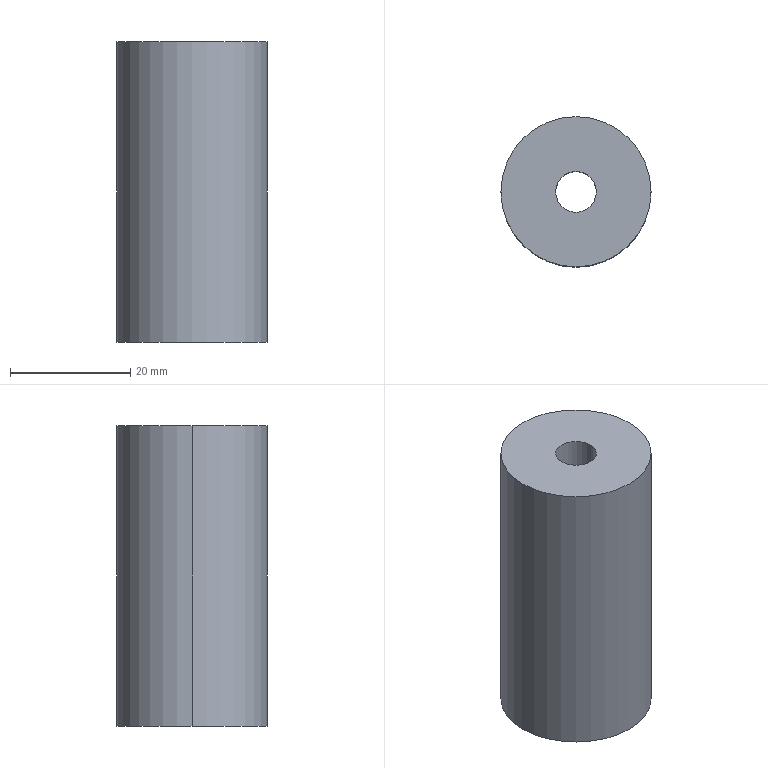Part | 1 solid | 6 faces | box 25 x 25 x 50 mm | volume 22728 mm3 | cylinder 4 | plane 2 | commonest cylinder face diameters 6.8 x2 25 x2
STEP:
#1=CARTESIAN_POINT('',(-3.4,0.,0.));
#2=VERTEX_POINT('',#1);
#3=CARTESIAN_POINT('',(3.4,0.,0.));
#4=VERTEX_POINT('',#3);
#5=CARTESIAN_POINT('',(0.,0.,0.));
#6=DIRECTION('',(0.,0.,1.));
#7=DIRECTION('',(1.,0.,0.));
#8=AXIS2_PLACEMENT_3D('',#5,#6,#7);
#9=CIRCLE('',#8,3.4);
#10=EDGE_CURVE('',#2,#4,#9,.T.);
#11=ORIENTED_EDGE('',*,*,#10,.F.);
#12=CARTESIAN_POINT('',(-3.4,0.,50.));
#13=VERTEX_POINT('',#12);
#14=CARTESIAN_POINT('',(-3.4,0.,50.));
#15=DIRECTION('',(0.,0.,1.));
#16=VECTOR('',#15,1000.);
#17=LINE('',#14,#16);
#18=EDGE_CURVE('',#2,#13,#17,.T.);
#19=ORIENTED_EDGE('',*,*,#18,.T.);
#20=CARTESIAN_POINT('',(3.4,0.,50.));
#21=VERTEX_POINT('',#20);
#22=CARTESIAN_POINT('',(0.,0.,50.));
#23=DIRECTION('',(0.,0.,1.));
#24=DIRECTION('',(1.,0.,0.));
#25=AXIS2_PLACEMENT_3D('',#22,#23,#24);
#26=CIRCLE('',#25,3.4);
#27=EDGE_CURVE('',#13,#21,#26,.T.);
#28=ORIENTED_EDGE('',*,*,#27,.T.);
#29=CARTESIAN_POINT('',(3.4,0.,50.));
#30=DIRECTION('',(0.,0.,1.));
#31=VECTOR('',#30,1000.);
#32=LINE('',#29,#31);
#33=EDGE_CURVE('',#4,#21,#32,.T.);
#34=ORIENTED_EDGE('',*,*,#33,.F.);
#35=EDGE_LOOP('',(#11,#19,#28,#34));
#36=FACE_OUTER_BOUND('',#35,.T.);
#37=CARTESIAN_POINT('',(0.,0.,50.));
#38=DIRECTION('',(0.,0.,1.));
#39=DIRECTION('',(1.,0.,0.));
#40=AXIS2_PLACEMENT_3D('',#37,#38,#39);
#41=CYLINDRICAL_SURFACE('',#40,3.4);
#42=ADVANCED_FACE('',(#36),#41,.F.);
#43=CARTESIAN_POINT('',(12.5,0.,50.));
#44=VERTEX_POINT('',#43);
#45=CARTESIAN_POINT('',(-12.5,0.,50.));
#46=VERTEX_POINT('',#45);
#47=CARTESIAN_POINT('',(0.,0.,50.));
#48=DIRECTION('',(0.,0.,1.));
#49=DIRECTION('',(1.,0.,0.));
#50=AXIS2_PLACEMENT_3D('',#47,#48,#49);
#51=CIRCLE('',#50,12.5);
#52=EDGE_CURVE('',#44,#46,#51,.T.);
#53=ORIENTED_EDGE('',*,*,#52,.F.);
#54=CARTESIAN_POINT('',(12.5,0.,0.));
#55=VERTEX_POINT('',#54);
#56=CARTESIAN_POINT('',(12.5,0.,50.));
#57=DIRECTION('',(0.,0.,-1.));
#58=VECTOR('',#57,1000.);
#59=LINE('',#56,#58);
#60=EDGE_CURVE('',#44,#55,#59,.T.);
#61=ORIENTED_EDGE('',*,*,#60,.T.);
#62=CARTESIAN_POINT('',(-12.5,0.,0.));
#63=VERTEX_POINT('',#62);
#64=CARTESIAN_POINT('',(0.,0.,0.));
#65=DIRECTION('',(0.,0.,1.));
#66=DIRECTION('',(1.,0.,0.));
#67=AXIS2_PLACEMENT_3D('',#64,#65,#66);
#68=CIRCLE('',#67,12.5);
#69=EDGE_CURVE('',#55,#63,#68,.T.);
#70=ORIENTED_EDGE('',*,*,#69,.T.);
#71=CARTESIAN_POINT('',(-12.5,0.,50.));
#72=DIRECTION('',(0.,0.,-1.));
#73=VECTOR('',#72,1000.);
#74=LINE('',#71,#73);
#75=EDGE_CURVE('',#46,#63,#74,.T.);
#76=ORIENTED_EDGE('',*,*,#75,.F.);
#77=EDGE_LOOP('',(#53,#61,#70,#76));
#78=FACE_OUTER_BOUND('',#77,.T.);
#79=CARTESIAN_POINT('',(0.,0.,50.));
#80=DIRECTION('',(0.,0.,-1.));
#81=DIRECTION('',(-1.,0.,0.));
#82=AXIS2_PLACEMENT_3D('',#79,#80,#81);
#83=CYLINDRICAL_SURFACE('',#82,12.5);
#84=ADVANCED_FACE('',(#78),#83,.T.);
#85=ORIENTED_EDGE('',*,*,#60,.F.);
#86=CARTESIAN_POINT('',(0.,0.,50.));
#87=DIRECTION('',(0.,0.,1.));
#88=DIRECTION('',(1.,0.,0.));
#89=AXIS2_PLACEMENT_3D('',#86,#87,#88);
#90=CIRCLE('',#89,12.5);
#91=EDGE_CURVE('',#46,#44,#90,.T.);
#92=ORIENTED_EDGE('',*,*,#91,.F.);
#93=ORIENTED_EDGE('',*,*,#75,.T.);
#94=CARTESIAN_POINT('',(0.,0.,0.));
#95=DIRECTION('',(0.,0.,1.));
#96=DIRECTION('',(1.,0.,0.));
#97=AXIS2_PLACEMENT_3D('',#94,#95,#96);
#98=CIRCLE('',#97,12.5);
#99=EDGE_CURVE('',#63,#55,#98,.T.);
#100=ORIENTED_EDGE('',*,*,#99,.T.);
#101=EDGE_LOOP('',(#85,#92,#93,#100));
#102=FACE_OUTER_BOUND('',#101,.T.);
#103=CARTESIAN_POINT('',(0.,0.,50.));
#104=DIRECTION('',(0.,0.,-1.));
#105=DIRECTION('',(-1.,0.,0.));
#106=AXIS2_PLACEMENT_3D('',#103,#104,#105);
#107=CYLINDRICAL_SURFACE('',#106,12.5);
#108=ADVANCED_FACE('',(#102),#107,.T.);
#109=CARTESIAN_POINT('',(0.,0.,50.));
#110=DIRECTION('',(0.,0.,1.));
#111=DIRECTION('',(1.,0.,0.));
#112=AXIS2_PLACEMENT_3D('',#109,#110,#111);
#113=CIRCLE('',#112,3.4);
#114=EDGE_CURVE('',#21,#13,#113,.T.);
#115=ORIENTED_EDGE('',*,*,#114,.F.);
#116=ORIENTED_EDGE('',*,*,#27,.F.);
#117=EDGE_LOOP('',(#115,#116));
#118=FACE_BOUND('',#117,.T.);
#119=ORIENTED_EDGE('',*,*,#91,.T.);
#120=ORIENTED_EDGE('',*,*,#52,.T.);
#121=EDGE_LOOP('',(#119,#120));
#122=FACE_OUTER_BOUND('',#121,.T.);
#123=CARTESIAN_POINT('',(0.,0.,50.));
#124=DIRECTION('',(0.,0.,1.));
#125=DIRECTION('',(1.,0.,0.));
#126=AXIS2_PLACEMENT_3D('',#123,#124,#125);
#127=PLANE('',#126);
#128=ADVANCED_FACE('',(#118,#122),#127,.T.);
#129=CARTESIAN_POINT('',(0.,0.,0.));
#130=DIRECTION('',(0.,0.,1.));
#131=DIRECTION('',(1.,0.,0.));
#132=AXIS2_PLACEMENT_3D('',#129,#130,#131);
#133=CIRCLE('',#132,3.4);
#134=EDGE_CURVE('',#4,#2,#133,.T.);
#135=ORIENTED_EDGE('',*,*,#134,.T.);
#136=ORIENTED_EDGE('',*,*,#10,.T.);
#137=EDGE_LOOP('',(#135,#136));
#138=FACE_BOUND('',#137,.T.);
#139=ORIENTED_EDGE('',*,*,#99,.F.);
#140=ORIENTED_EDGE('',*,*,#69,.F.);
#141=EDGE_LOOP('',(#139,#140));
#142=FACE_OUTER_BOUND('',#141,.T.);
#143=CARTESIAN_POINT('',(0.,0.,0.));
#144=DIRECTION('',(0.,0.,1.));
#145=DIRECTION('',(1.,0.,0.));
#146=AXIS2_PLACEMENT_3D('',#143,#144,#145);
#147=PLANE('',#146);
#148=ADVANCED_FACE('',(#138,#142),#147,.F.);
#149=ORIENTED_EDGE('',*,*,#18,.F.);
#150=ORIENTED_EDGE('',*,*,#134,.F.);
#151=ORIENTED_EDGE('',*,*,#33,.T.);
#152=ORIENTED_EDGE('',*,*,#114,.T.);
#153=EDGE_LOOP('',(#149,#150,#151,#152));
#154=FACE_OUTER_BOUND('',#153,.T.);
#155=CARTESIAN_POINT('',(0.,0.,50.));
#156=DIRECTION('',(0.,0.,1.));
#157=DIRECTION('',(1.,0.,0.));
#158=AXIS2_PLACEMENT_3D('',#155,#156,#157);
#159=CYLINDRICAL_SURFACE('',#158,3.4);
#160=ADVANCED_FACE('',(#154),#159,.F.);
#161=CLOSED_SHELL('',(#42,#84,#108,#128,#148,#160));
#162=MANIFOLD_SOLID_BREP('',#161);
#163=CARTESIAN_POINT('',(0.,0.,0.));
#164=DIRECTION('',(0.,0.,1.));
#165=DIRECTION('',(1.,0.,0.));
#166=AXIS2_PLACEMENT_3D('',#163,#164,#165);
#167=(LENGTH_UNIT()NAMED_UNIT(*)SI_UNIT(.MILLI.,.METRE.));
#168=UNCERTAINTY_MEASURE_WITH_UNIT(LENGTH_MEASURE(0.00001),#167,'','');
#169=(NAMED_UNIT(*)PLANE_ANGLE_UNIT()SI_UNIT($,.RADIAN.));
#170=(NAMED_UNIT(*)SI_UNIT($,.STERADIAN.)SOLID_ANGLE_UNIT());
#171=(GEOMETRIC_REPRESENTATION_CONTEXT(3)GLOBAL_UNCERTAINTY_ASSIGNED_CONTEXT((#168))GLOBAL_UNIT_ASSIGNED_CONTEXT((#167,#169,#170))REPRESENTATION_CONTEXT('',''));
#172=ADVANCED_BREP_SHAPE_REPRESENTATION('',(#162,#166),#171);